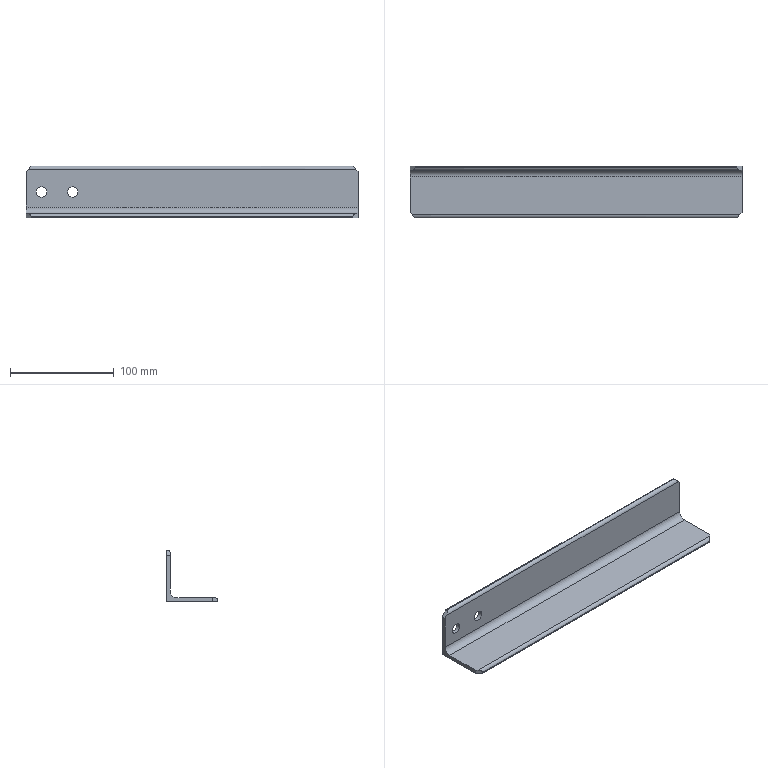Part | STEP file | [03]-7 | 1 solid | 19 faces | box 320 x 50 x 50 mm | volume 123750 mm3 | plane 12 | cylinder 7 | commonest cylinder face diameters 10 x4 6 x2 13 x1